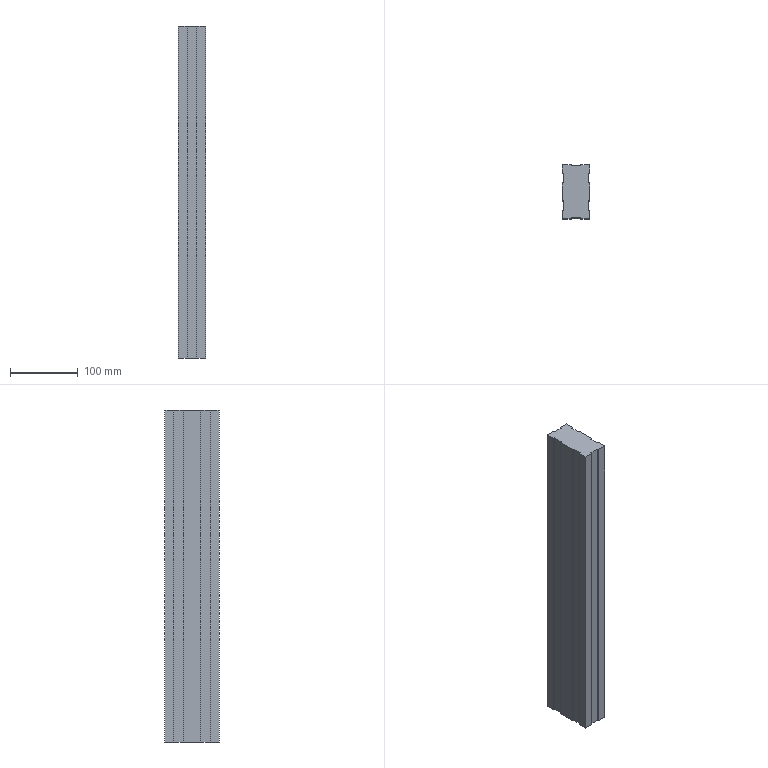Part | STEP file | xingcai40x80x490 | 1 solid | 30 faces | box 40 x 80 x 490 mm | volume 1485680 mm3 | plane 30